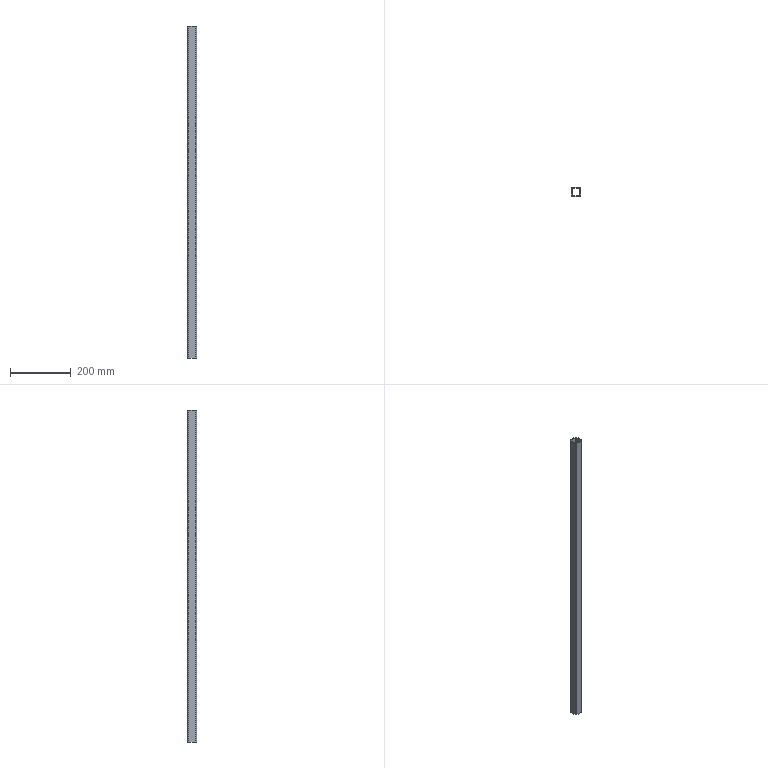Part | SolidWorks | features Attribute 1, ExtruThin 1 | 1 solid | 18 faces | box 30 x 30 x 1098 mm | volume 234556 mm3 | plane 10 | cylinder 8 | commonest cylinder face diameters 4 x4 8 x4
STEP:
#1=CARTESIAN_POINT('',(15.,11.,548.8));
#2=VERTEX_POINT('',#1);
#3=CARTESIAN_POINT('',(11.,15.,548.8));
#4=VERTEX_POINT('',#3);
#5=CARTESIAN_POINT('',(11.,11.,548.8));
#6=DIRECTION('',(0.,0.,1.));
#7=DIRECTION('',(1.,0.,0.));
#8=AXIS2_PLACEMENT_3D('',#5,#6,#7);
#9=CIRCLE('',#8,4.);
#10=EDGE_CURVE('',#2,#4,#9,.T.);
#11=ORIENTED_EDGE('',*,*,#10,.T.);
#12=CARTESIAN_POINT('',(-11.,15.,548.8));
#13=VERTEX_POINT('',#12);
#14=CARTESIAN_POINT('',(11.,15.,548.8));
#15=DIRECTION('',(-1.,0.,0.));
#16=VECTOR('',#15,1000.);
#17=LINE('',#14,#16);
#18=EDGE_CURVE('',#4,#13,#17,.T.);
#19=ORIENTED_EDGE('',*,*,#18,.T.);
#20=CARTESIAN_POINT('',(-15.,11.,548.8));
#21=VERTEX_POINT('',#20);
#22=CARTESIAN_POINT('',(-11.,11.,548.8));
#23=DIRECTION('',(0.,0.,1.));
#24=DIRECTION('',(1.,0.,0.));
#25=AXIS2_PLACEMENT_3D('',#22,#23,#24);
#26=CIRCLE('',#25,4.);
#27=EDGE_CURVE('',#13,#21,#26,.T.);
#28=ORIENTED_EDGE('',*,*,#27,.T.);
#29=CARTESIAN_POINT('',(-15.,-11.,548.8));
#30=VERTEX_POINT('',#29);
#31=CARTESIAN_POINT('',(-15.,-11.,548.8));
#32=DIRECTION('',(0.,1.,0.));
#33=VECTOR('',#32,1000.);
#34=LINE('',#31,#33);
#35=EDGE_CURVE('',#30,#21,#34,.T.);
#36=ORIENTED_EDGE('',*,*,#35,.F.);
#37=CARTESIAN_POINT('',(-11.,-15.,548.8));
#38=VERTEX_POINT('',#37);
#39=CARTESIAN_POINT('',(-11.,-11.,548.8));
#40=DIRECTION('',(0.,0.,1.));
#41=DIRECTION('',(1.,0.,0.));
#42=AXIS2_PLACEMENT_3D('',#39,#40,#41);
#43=CIRCLE('',#42,4.);
#44=EDGE_CURVE('',#30,#38,#43,.T.);
#45=ORIENTED_EDGE('',*,*,#44,.T.);
#46=CARTESIAN_POINT('',(11.,-15.,548.8));
#47=VERTEX_POINT('',#46);
#48=CARTESIAN_POINT('',(-11.,-15.,548.8));
#49=DIRECTION('',(1.,0.,0.));
#50=VECTOR('',#49,1000.);
#51=LINE('',#48,#50);
#52=EDGE_CURVE('',#38,#47,#51,.T.);
#53=ORIENTED_EDGE('',*,*,#52,.T.);
#54=CARTESIAN_POINT('',(15.,-11.,548.8));
#55=VERTEX_POINT('',#54);
#56=CARTESIAN_POINT('',(11.,-11.,548.8));
#57=DIRECTION('',(0.,0.,1.));
#58=DIRECTION('',(1.,0.,0.));
#59=AXIS2_PLACEMENT_3D('',#56,#57,#58);
#60=CIRCLE('',#59,4.);
#61=EDGE_CURVE('',#47,#55,#60,.T.);
#62=ORIENTED_EDGE('',*,*,#61,.T.);
#63=CARTESIAN_POINT('',(15.,11.,548.8));
#64=DIRECTION('',(0.,-1.,0.));
#65=VECTOR('',#64,1000.);
#66=LINE('',#63,#65);
#67=EDGE_CURVE('',#2,#55,#66,.T.);
#68=ORIENTED_EDGE('',*,*,#67,.F.);
#69=EDGE_LOOP('',(#11,#19,#28,#36,#45,#53,#62,#68));
#70=FACE_OUTER_BOUND('',#69,.T.);
#71=CARTESIAN_POINT('',(11.,13.,548.8));
#72=VERTEX_POINT('',#71);
#73=CARTESIAN_POINT('',(-11.,13.,548.8));
#74=VERTEX_POINT('',#73);
#75=CARTESIAN_POINT('',(11.,13.,548.8));
#76=DIRECTION('',(-1.,0.,0.));
#77=VECTOR('',#76,1000.);
#78=LINE('',#75,#77);
#79=EDGE_CURVE('',#72,#74,#78,.T.);
#80=ORIENTED_EDGE('',*,*,#79,.F.);
#81=CARTESIAN_POINT('',(13.,11.,548.8));
#82=VERTEX_POINT('',#81);
#83=CARTESIAN_POINT('',(11.,11.,548.8));
#84=DIRECTION('',(0.,0.,1.));
#85=DIRECTION('',(1.,0.,0.));
#86=AXIS2_PLACEMENT_3D('',#83,#84,#85);
#87=CIRCLE('',#86,2.);
#88=EDGE_CURVE('',#82,#72,#87,.T.);
#89=ORIENTED_EDGE('',*,*,#88,.F.);
#90=CARTESIAN_POINT('',(13.,-11.,548.8));
#91=VERTEX_POINT('',#90);
#92=CARTESIAN_POINT('',(13.,11.,548.8));
#93=DIRECTION('',(0.,-1.,0.));
#94=VECTOR('',#93,1000.);
#95=LINE('',#92,#94);
#96=EDGE_CURVE('',#82,#91,#95,.T.);
#97=ORIENTED_EDGE('',*,*,#96,.T.);
#98=CARTESIAN_POINT('',(11.,-13.,548.8));
#99=VERTEX_POINT('',#98);
#100=CARTESIAN_POINT('',(11.,-11.,548.8));
#101=DIRECTION('',(0.,0.,1.));
#102=DIRECTION('',(1.,0.,0.));
#103=AXIS2_PLACEMENT_3D('',#100,#101,#102);
#104=CIRCLE('',#103,2.);
#105=EDGE_CURVE('',#99,#91,#104,.T.);
#106=ORIENTED_EDGE('',*,*,#105,.F.);
#107=CARTESIAN_POINT('',(-11.,-13.,548.8));
#108=VERTEX_POINT('',#107);
#109=CARTESIAN_POINT('',(-11.,-13.,548.8));
#110=DIRECTION('',(1.,0.,0.));
#111=VECTOR('',#110,1000.);
#112=LINE('',#109,#111);
#113=EDGE_CURVE('',#108,#99,#112,.T.);
#114=ORIENTED_EDGE('',*,*,#113,.F.);
#115=CARTESIAN_POINT('',(-13.,-11.,548.8));
#116=VERTEX_POINT('',#115);
#117=CARTESIAN_POINT('',(-11.,-11.,548.8));
#118=DIRECTION('',(0.,0.,1.));
#119=DIRECTION('',(1.,0.,0.));
#120=AXIS2_PLACEMENT_3D('',#117,#118,#119);
#121=CIRCLE('',#120,2.);
#122=EDGE_CURVE('',#116,#108,#121,.T.);
#123=ORIENTED_EDGE('',*,*,#122,.F.);
#124=CARTESIAN_POINT('',(-13.,11.,548.8));
#125=VERTEX_POINT('',#124);
#126=CARTESIAN_POINT('',(-13.,-11.,548.8));
#127=DIRECTION('',(0.,1.,0.));
#128=VECTOR('',#127,1000.);
#129=LINE('',#126,#128);
#130=EDGE_CURVE('',#116,#125,#129,.T.);
#131=ORIENTED_EDGE('',*,*,#130,.T.);
#132=CARTESIAN_POINT('',(-11.,11.,548.8));
#133=DIRECTION('',(0.,0.,1.));
#134=DIRECTION('',(1.,0.,0.));
#135=AXIS2_PLACEMENT_3D('',#132,#133,#134);
#136=CIRCLE('',#135,2.);
#137=EDGE_CURVE('',#74,#125,#136,.T.);
#138=ORIENTED_EDGE('',*,*,#137,.F.);
#139=EDGE_LOOP('',(#80,#89,#97,#106,#114,#123,#131,#138));
#140=FACE_BOUND('',#139,.T.);
#141=CARTESIAN_POINT('',(11.,11.,548.8));
#142=DIRECTION('',(0.,0.,1.));
#143=DIRECTION('',(1.,0.,0.));
#144=AXIS2_PLACEMENT_3D('',#141,#142,#143);
#145=PLANE('',#144);
#146=ADVANCED_FACE('',(#70,#140),#145,.T.);
#147=CARTESIAN_POINT('',(15.,11.,-548.8));
#148=VERTEX_POINT('',#147);
#149=CARTESIAN_POINT('',(11.,15.,-548.8));
#150=VERTEX_POINT('',#149);
#151=CARTESIAN_POINT('',(11.,11.,-548.8));
#152=DIRECTION('',(0.,0.,1.));
#153=DIRECTION('',(1.,0.,0.));
#154=AXIS2_PLACEMENT_3D('',#151,#152,#153);
#155=CIRCLE('',#154,4.);
#156=EDGE_CURVE('',#148,#150,#155,.T.);
#157=ORIENTED_EDGE('',*,*,#156,.F.);
#158=CARTESIAN_POINT('',(15.,-11.,-548.8));
#159=VERTEX_POINT('',#158);
#160=CARTESIAN_POINT('',(15.,11.,-548.8));
#161=DIRECTION('',(0.,-1.,0.));
#162=VECTOR('',#161,1000.);
#163=LINE('',#160,#162);
#164=EDGE_CURVE('',#148,#159,#163,.T.);
#165=ORIENTED_EDGE('',*,*,#164,.T.);
#166=CARTESIAN_POINT('',(11.,-15.,-548.8));
#167=VERTEX_POINT('',#166);
#168=CARTESIAN_POINT('',(11.,-11.,-548.8));
#169=DIRECTION('',(0.,0.,1.));
#170=DIRECTION('',(1.,0.,0.));
#171=AXIS2_PLACEMENT_3D('',#168,#169,#170);
#172=CIRCLE('',#171,4.);
#173=EDGE_CURVE('',#167,#159,#172,.T.);
#174=ORIENTED_EDGE('',*,*,#173,.F.);
#175=CARTESIAN_POINT('',(-11.,-15.,-548.8));
#176=VERTEX_POINT('',#175);
#177=CARTESIAN_POINT('',(-11.,-15.,-548.8));
#178=DIRECTION('',(1.,0.,0.));
#179=VECTOR('',#178,1000.);
#180=LINE('',#177,#179);
#181=EDGE_CURVE('',#176,#167,#180,.T.);
#182=ORIENTED_EDGE('',*,*,#181,.F.);
#183=CARTESIAN_POINT('',(-15.,-11.,-548.8));
#184=VERTEX_POINT('',#183);
#185=CARTESIAN_POINT('',(-11.,-11.,-548.8));
#186=DIRECTION('',(0.,0.,1.));
#187=DIRECTION('',(1.,0.,0.));
#188=AXIS2_PLACEMENT_3D('',#185,#186,#187);
#189=CIRCLE('',#188,4.);
#190=EDGE_CURVE('',#184,#176,#189,.T.);
#191=ORIENTED_EDGE('',*,*,#190,.F.);
#192=CARTESIAN_POINT('',(-15.,11.,-548.8));
#193=VERTEX_POINT('',#192);
#194=CARTESIAN_POINT('',(-15.,-11.,-548.8));
#195=DIRECTION('',(0.,1.,0.));
#196=VECTOR('',#195,1000.);
#197=LINE('',#194,#196);
#198=EDGE_CURVE('',#184,#193,#197,.T.);
#199=ORIENTED_EDGE('',*,*,#198,.T.);
#200=CARTESIAN_POINT('',(-11.,15.,-548.8));
#201=VERTEX_POINT('',#200);
#202=CARTESIAN_POINT('',(-11.,11.,-548.8));
#203=DIRECTION('',(0.,0.,1.));
#204=DIRECTION('',(1.,0.,0.));
#205=AXIS2_PLACEMENT_3D('',#202,#203,#204);
#206=CIRCLE('',#205,4.);
#207=EDGE_CURVE('',#201,#193,#206,.T.);
#208=ORIENTED_EDGE('',*,*,#207,.F.);
#209=CARTESIAN_POINT('',(11.,15.,-548.8));
#210=DIRECTION('',(-1.,0.,0.));
#211=VECTOR('',#210,1000.);
#212=LINE('',#209,#211);
#213=EDGE_CURVE('',#150,#201,#212,.T.);
#214=ORIENTED_EDGE('',*,*,#213,.F.);
#215=EDGE_LOOP('',(#157,#165,#174,#182,#191,#199,#208,#214));
#216=FACE_OUTER_BOUND('',#215,.T.);
#217=CARTESIAN_POINT('',(13.,11.,-548.8));
#218=VERTEX_POINT('',#217);
#219=CARTESIAN_POINT('',(11.,13.,-548.8));
#220=VERTEX_POINT('',#219);
#221=CARTESIAN_POINT('',(11.,11.,-548.8));
#222=DIRECTION('',(0.,0.,1.));
#223=DIRECTION('',(1.,0.,0.));
#224=AXIS2_PLACEMENT_3D('',#221,#222,#223);
#225=CIRCLE('',#224,2.);
#226=EDGE_CURVE('',#218,#220,#225,.T.);
#227=ORIENTED_EDGE('',*,*,#226,.T.);
#228=CARTESIAN_POINT('',(-11.,13.,-548.8));
#229=VERTEX_POINT('',#228);
#230=CARTESIAN_POINT('',(11.,13.,-548.8));
#231=DIRECTION('',(-1.,0.,0.));
#232=VECTOR('',#231,1000.);
#233=LINE('',#230,#232);
#234=EDGE_CURVE('',#220,#229,#233,.T.);
#235=ORIENTED_EDGE('',*,*,#234,.T.);
#236=CARTESIAN_POINT('',(-13.,11.,-548.8));
#237=VERTEX_POINT('',#236);
#238=CARTESIAN_POINT('',(-11.,11.,-548.8));
#239=DIRECTION('',(0.,0.,1.));
#240=DIRECTION('',(1.,0.,0.));
#241=AXIS2_PLACEMENT_3D('',#238,#239,#240);
#242=CIRCLE('',#241,2.);
#243=EDGE_CURVE('',#229,#237,#242,.T.);
#244=ORIENTED_EDGE('',*,*,#243,.T.);
#245=CARTESIAN_POINT('',(-13.,-11.,-548.8));
#246=VERTEX_POINT('',#245);
#247=CARTESIAN_POINT('',(-13.,-11.,-548.8));
#248=DIRECTION('',(0.,1.,0.));
#249=VECTOR('',#248,1000.);
#250=LINE('',#247,#249);
#251=EDGE_CURVE('',#246,#237,#250,.T.);
#252=ORIENTED_EDGE('',*,*,#251,.F.);
#253=CARTESIAN_POINT('',(-11.,-13.,-548.8));
#254=VERTEX_POINT('',#253);
#255=CARTESIAN_POINT('',(-11.,-11.,-548.8));
#256=DIRECTION('',(0.,0.,1.));
#257=DIRECTION('',(1.,0.,0.));
#258=AXIS2_PLACEMENT_3D('',#255,#256,#257);
#259=CIRCLE('',#258,2.);
#260=EDGE_CURVE('',#246,#254,#259,.T.);
#261=ORIENTED_EDGE('',*,*,#260,.T.);
#262=CARTESIAN_POINT('',(11.,-13.,-548.8));
#263=VERTEX_POINT('',#262);
#264=CARTESIAN_POINT('',(-11.,-13.,-548.8));
#265=DIRECTION('',(1.,0.,0.));
#266=VECTOR('',#265,1000.);
#267=LINE('',#264,#266);
#268=EDGE_CURVE('',#254,#263,#267,.T.);
#269=ORIENTED_EDGE('',*,*,#268,.T.);
#270=CARTESIAN_POINT('',(13.,-11.,-548.8));
#271=VERTEX_POINT('',#270);
#272=CARTESIAN_POINT('',(11.,-11.,-548.8));
#273=DIRECTION('',(0.,0.,1.));
#274=DIRECTION('',(1.,0.,0.));
#275=AXIS2_PLACEMENT_3D('',#272,#273,#274);
#276=CIRCLE('',#275,2.);
#277=EDGE_CURVE('',#263,#271,#276,.T.);
#278=ORIENTED_EDGE('',*,*,#277,.T.);
#279=CARTESIAN_POINT('',(13.,11.,-548.8));
#280=DIRECTION('',(0.,-1.,0.));
#281=VECTOR('',#280,1000.);
#282=LINE('',#279,#281);
#283=EDGE_CURVE('',#218,#271,#282,.T.);
#284=ORIENTED_EDGE('',*,*,#283,.F.);
#285=EDGE_LOOP('',(#227,#235,#244,#252,#261,#269,#278,#284));
#286=FACE_BOUND('',#285,.T.);
#287=CARTESIAN_POINT('',(11.,11.,-548.8));
#288=DIRECTION('',(0.,0.,1.));
#289=DIRECTION('',(1.,0.,0.));
#290=AXIS2_PLACEMENT_3D('',#287,#288,#289);
#291=PLANE('',#290);
#292=ADVANCED_FACE('',(#216,#286),#291,.F.);
#293=ORIENTED_EDGE('',*,*,#156,.T.);
#294=CARTESIAN_POINT('',(11.,15.,548.8));
#295=DIRECTION('',(0.,0.,-1.));
#296=VECTOR('',#295,1000.);
#297=LINE('',#294,#296);
#298=EDGE_CURVE('',#4,#150,#297,.T.);
#299=ORIENTED_EDGE('',*,*,#298,.F.);
#300=ORIENTED_EDGE('',*,*,#10,.F.);
#301=CARTESIAN_POINT('',(15.,11.,548.8));
#302=DIRECTION('',(0.,0.,-1.));
#303=VECTOR('',#302,1000.);
#304=LINE('',#301,#303);
#305=EDGE_CURVE('',#2,#148,#304,.T.);
#306=ORIENTED_EDGE('',*,*,#305,.T.);
#307=EDGE_LOOP('',(#293,#299,#300,#306));
#308=FACE_OUTER_BOUND('',#307,.T.);
#309=CARTESIAN_POINT('',(11.,11.,548.8));
#310=DIRECTION('',(0.,0.,-1.));
#311=DIRECTION('',(-1.,0.,0.));
#312=AXIS2_PLACEMENT_3D('',#309,#310,#311);
#313=CYLINDRICAL_SURFACE('',#312,4.);
#314=ADVANCED_FACE('',(#308),#313,.T.);
#315=ORIENTED_EDGE('',*,*,#213,.T.);
#316=CARTESIAN_POINT('',(-11.,15.,548.8));
#317=DIRECTION('',(0.,0.,-1.));
#318=VECTOR('',#317,1000.);
#319=LINE('',#316,#318);
#320=EDGE_CURVE('',#13,#201,#319,.T.);
#321=ORIENTED_EDGE('',*,*,#320,.F.);
#322=ORIENTED_EDGE('',*,*,#18,.F.);
#323=ORIENTED_EDGE('',*,*,#298,.T.);
#324=EDGE_LOOP('',(#315,#321,#322,#323));
#325=FACE_OUTER_BOUND('',#324,.T.);
#326=CARTESIAN_POINT('',(11.,15.,548.8));
#327=DIRECTION('',(0.,-1.,0.));
#328=DIRECTION('',(0.,0.,-1.));
#329=AXIS2_PLACEMENT_3D('',#326,#327,#328);
#330=PLANE('',#329);
#331=ADVANCED_FACE('',(#325),#330,.F.);
#332=ORIENTED_EDGE('',*,*,#207,.T.);
#333=CARTESIAN_POINT('',(-15.,11.,548.8));
#334=DIRECTION('',(0.,0.,-1.));
#335=VECTOR('',#334,1000.);
#336=LINE('',#333,#335);
#337=EDGE_CURVE('',#21,#193,#336,.T.);
#338=ORIENTED_EDGE('',*,*,#337,.F.);
#339=ORIENTED_EDGE('',*,*,#27,.F.);
#340=ORIENTED_EDGE('',*,*,#320,.T.);
#341=EDGE_LOOP('',(#332,#338,#339,#340));
#342=FACE_OUTER_BOUND('',#341,.T.);
#343=CARTESIAN_POINT('',(-11.,11.,548.8));
#344=DIRECTION('',(0.,0.,-1.));
#345=DIRECTION('',(-1.,0.,0.));
#346=AXIS2_PLACEMENT_3D('',#343,#344,#345);
#347=CYLINDRICAL_SURFACE('',#346,4.);
#348=ADVANCED_FACE('',(#342),#347,.T.);
#349=ORIENTED_EDGE('',*,*,#198,.F.);
#350=CARTESIAN_POINT('',(-15.,-11.,548.8));
#351=DIRECTION('',(0.,0.,-1.));
#352=VECTOR('',#351,1000.);
#353=LINE('',#350,#352);
#354=EDGE_CURVE('',#30,#184,#353,.T.);
#355=ORIENTED_EDGE('',*,*,#354,.F.);
#356=ORIENTED_EDGE('',*,*,#35,.T.);
#357=ORIENTED_EDGE('',*,*,#337,.T.);
#358=EDGE_LOOP('',(#349,#355,#356,#357));
#359=FACE_OUTER_BOUND('',#358,.T.);
#360=CARTESIAN_POINT('',(-15.,-11.,548.8));
#361=DIRECTION('',(-1.,0.,0.));
#362=DIRECTION('',(0.,0.,1.));
#363=AXIS2_PLACEMENT_3D('',#360,#361,#362);
#364=PLANE('',#363);
#365=ADVANCED_FACE('',(#359),#364,.T.);
#366=ORIENTED_EDGE('',*,*,#190,.T.);
#367=CARTESIAN_POINT('',(-11.,-15.,548.8));
#368=DIRECTION('',(0.,0.,-1.));
#369=VECTOR('',#368,1000.);
#370=LINE('',#367,#369);
#371=EDGE_CURVE('',#38,#176,#370,.T.);
#372=ORIENTED_EDGE('',*,*,#371,.F.);
#373=ORIENTED_EDGE('',*,*,#44,.F.);
#374=ORIENTED_EDGE('',*,*,#354,.T.);
#375=EDGE_LOOP('',(#366,#372,#373,#374));
#376=FACE_OUTER_BOUND('',#375,.T.);
#377=CARTESIAN_POINT('',(-11.,-11.,548.8));
#378=DIRECTION('',(0.,0.,-1.));
#379=DIRECTION('',(-1.,0.,0.));
#380=AXIS2_PLACEMENT_3D('',#377,#378,#379);
#381=CYLINDRICAL_SURFACE('',#380,4.);
#382=ADVANCED_FACE('',(#376),#381,.T.);
#383=ORIENTED_EDGE('',*,*,#181,.T.);
#384=CARTESIAN_POINT('',(11.,-15.,548.8));
#385=DIRECTION('',(0.,0.,-1.));
#386=VECTOR('',#385,1000.);
#387=LINE('',#384,#386);
#388=EDGE_CURVE('',#47,#167,#387,.T.);
#389=ORIENTED_EDGE('',*,*,#388,.F.);
#390=ORIENTED_EDGE('',*,*,#52,.F.);
#391=ORIENTED_EDGE('',*,*,#371,.T.);
#392=EDGE_LOOP('',(#383,#389,#390,#391));
#393=FACE_OUTER_BOUND('',#392,.T.);
#394=CARTESIAN_POINT('',(-11.,-15.,548.8));
#395=DIRECTION('',(0.,1.,0.));
#396=DIRECTION('',(0.,0.,1.));
#397=AXIS2_PLACEMENT_3D('',#394,#395,#396);
#398=PLANE('',#397);
#399=ADVANCED_FACE('',(#393),#398,.F.);
#400=ORIENTED_EDGE('',*,*,#173,.T.);
#401=CARTESIAN_POINT('',(15.,-11.,548.8));
#402=DIRECTION('',(0.,0.,-1.));
#403=VECTOR('',#402,1000.);
#404=LINE('',#401,#403);
#405=EDGE_CURVE('',#55,#159,#404,.T.);
#406=ORIENTED_EDGE('',*,*,#405,.F.);
#407=ORIENTED_EDGE('',*,*,#61,.F.);
#408=ORIENTED_EDGE('',*,*,#388,.T.);
#409=EDGE_LOOP('',(#400,#406,#407,#408));
#410=FACE_OUTER_BOUND('',#409,.T.);
#411=CARTESIAN_POINT('',(11.,-11.,548.8));
#412=DIRECTION('',(0.,0.,-1.));
#413=DIRECTION('',(-1.,0.,0.));
#414=AXIS2_PLACEMENT_3D('',#411,#412,#413);
#415=CYLINDRICAL_SURFACE('',#414,4.);
#416=ADVANCED_FACE('',(#410),#415,.T.);
#417=ORIENTED_EDGE('',*,*,#164,.F.);
#418=ORIENTED_EDGE('',*,*,#305,.F.);
#419=ORIENTED_EDGE('',*,*,#67,.T.);
#420=ORIENTED_EDGE('',*,*,#405,.T.);
#421=EDGE_LOOP('',(#417,#418,#419,#420));
#422=FACE_OUTER_BOUND('',#421,.T.);
#423=CARTESIAN_POINT('',(15.,11.,548.8));
#424=DIRECTION('',(1.,0.,0.));
#425=DIRECTION('',(0.,0.,-1.));
#426=AXIS2_PLACEMENT_3D('',#423,#424,#425);
#427=PLANE('',#426);
#428=ADVANCED_FACE('',(#422),#427,.T.);
#429=ORIENTED_EDGE('',*,*,#226,.F.);
#430=CARTESIAN_POINT('',(13.,11.,548.8));
#431=DIRECTION('',(0.,0.,-1.));
#432=VECTOR('',#431,1000.);
#433=LINE('',#430,#432);
#434=EDGE_CURVE('',#82,#218,#433,.T.);
#435=ORIENTED_EDGE('',*,*,#434,.F.);
#436=ORIENTED_EDGE('',*,*,#88,.T.);
#437=CARTESIAN_POINT('',(11.,13.,548.8));
#438=DIRECTION('',(0.,0.,-1.));
#439=VECTOR('',#438,1000.);
#440=LINE('',#437,#439);
#441=EDGE_CURVE('',#72,#220,#440,.T.);
#442=ORIENTED_EDGE('',*,*,#441,.T.);
#443=EDGE_LOOP('',(#429,#435,#436,#442));
#444=FACE_OUTER_BOUND('',#443,.T.);
#445=CARTESIAN_POINT('',(11.,11.,548.8));
#446=DIRECTION('',(0.,0.,-1.));
#447=DIRECTION('',(-1.,0.,0.));
#448=AXIS2_PLACEMENT_3D('',#445,#446,#447);
#449=CYLINDRICAL_SURFACE('',#448,2.);
#450=ADVANCED_FACE('',(#444),#449,.F.);
#451=ORIENTED_EDGE('',*,*,#234,.F.);
#452=ORIENTED_EDGE('',*,*,#441,.F.);
#453=ORIENTED_EDGE('',*,*,#79,.T.);
#454=CARTESIAN_POINT('',(-11.,13.,548.8));
#455=DIRECTION('',(0.,0.,-1.));
#456=VECTOR('',#455,1000.);
#457=LINE('',#454,#456);
#458=EDGE_CURVE('',#74,#229,#457,.T.);
#459=ORIENTED_EDGE('',*,*,#458,.T.);
#460=EDGE_LOOP('',(#451,#452,#453,#459));
#461=FACE_OUTER_BOUND('',#460,.T.);
#462=CARTESIAN_POINT('',(11.,13.,548.8));
#463=DIRECTION('',(0.,-1.,0.));
#464=DIRECTION('',(0.,0.,-1.));
#465=AXIS2_PLACEMENT_3D('',#462,#463,#464);
#466=PLANE('',#465);
#467=ADVANCED_FACE('',(#461),#466,.T.);
#468=ORIENTED_EDGE('',*,*,#243,.F.);
#469=ORIENTED_EDGE('',*,*,#458,.F.);
#470=ORIENTED_EDGE('',*,*,#137,.T.);
#471=CARTESIAN_POINT('',(-13.,11.,548.8));
#472=DIRECTION('',(0.,0.,-1.));
#473=VECTOR('',#472,1000.);
#474=LINE('',#471,#473);
#475=EDGE_CURVE('',#125,#237,#474,.T.);
#476=ORIENTED_EDGE('',*,*,#475,.T.);
#477=EDGE_LOOP('',(#468,#469,#470,#476));
#478=FACE_OUTER_BOUND('',#477,.T.);
#479=CARTESIAN_POINT('',(-11.,11.,548.8));
#480=DIRECTION('',(0.,0.,-1.));
#481=DIRECTION('',(-1.,0.,0.));
#482=AXIS2_PLACEMENT_3D('',#479,#480,#481);
#483=CYLINDRICAL_SURFACE('',#482,2.);
#484=ADVANCED_FACE('',(#478),#483,.F.);
#485=ORIENTED_EDGE('',*,*,#251,.T.);
#486=ORIENTED_EDGE('',*,*,#475,.F.);
#487=ORIENTED_EDGE('',*,*,#130,.F.);
#488=CARTESIAN_POINT('',(-13.,-11.,548.8));
#489=DIRECTION('',(0.,0.,-1.));
#490=VECTOR('',#489,1000.);
#491=LINE('',#488,#490);
#492=EDGE_CURVE('',#116,#246,#491,.T.);
#493=ORIENTED_EDGE('',*,*,#492,.T.);
#494=EDGE_LOOP('',(#485,#486,#487,#493));
#495=FACE_OUTER_BOUND('',#494,.T.);
#496=CARTESIAN_POINT('',(-13.,-11.,548.8));
#497=DIRECTION('',(-1.,0.,0.));
#498=DIRECTION('',(0.,0.,1.));
#499=AXIS2_PLACEMENT_3D('',#496,#497,#498);
#500=PLANE('',#499);
#501=ADVANCED_FACE('',(#495),#500,.F.);
#502=ORIENTED_EDGE('',*,*,#260,.F.);
#503=ORIENTED_EDGE('',*,*,#492,.F.);
#504=ORIENTED_EDGE('',*,*,#122,.T.);
#505=CARTESIAN_POINT('',(-11.,-13.,548.8));
#506=DIRECTION('',(0.,0.,-1.));
#507=VECTOR('',#506,1000.);
#508=LINE('',#505,#507);
#509=EDGE_CURVE('',#108,#254,#508,.T.);
#510=ORIENTED_EDGE('',*,*,#509,.T.);
#511=EDGE_LOOP('',(#502,#503,#504,#510));
#512=FACE_OUTER_BOUND('',#511,.T.);
#513=CARTESIAN_POINT('',(-11.,-11.,548.8));
#514=DIRECTION('',(0.,0.,-1.));
#515=DIRECTION('',(-1.,0.,0.));
#516=AXIS2_PLACEMENT_3D('',#513,#514,#515);
#517=CYLINDRICAL_SURFACE('',#516,2.);
#518=ADVANCED_FACE('',(#512),#517,.F.);
#519=ORIENTED_EDGE('',*,*,#268,.F.);
#520=ORIENTED_EDGE('',*,*,#509,.F.);
#521=ORIENTED_EDGE('',*,*,#113,.T.);
#522=CARTESIAN_POINT('',(11.,-13.,548.8));
#523=DIRECTION('',(0.,0.,-1.));
#524=VECTOR('',#523,1000.);
#525=LINE('',#522,#524);
#526=EDGE_CURVE('',#99,#263,#525,.T.);
#527=ORIENTED_EDGE('',*,*,#526,.T.);
#528=EDGE_LOOP('',(#519,#520,#521,#527));
#529=FACE_OUTER_BOUND('',#528,.T.);
#530=CARTESIAN_POINT('',(-11.,-13.,548.8));
#531=DIRECTION('',(0.,1.,0.));
#532=DIRECTION('',(0.,0.,1.));
#533=AXIS2_PLACEMENT_3D('',#530,#531,#532);
#534=PLANE('',#533);
#535=ADVANCED_FACE('',(#529),#534,.T.);
#536=ORIENTED_EDGE('',*,*,#277,.F.);
#537=ORIENTED_EDGE('',*,*,#526,.F.);
#538=ORIENTED_EDGE('',*,*,#105,.T.);
#539=CARTESIAN_POINT('',(13.,-11.,548.8));
#540=DIRECTION('',(0.,0.,-1.));
#541=VECTOR('',#540,1000.);
#542=LINE('',#539,#541);
#543=EDGE_CURVE('',#91,#271,#542,.T.);
#544=ORIENTED_EDGE('',*,*,#543,.T.);
#545=EDGE_LOOP('',(#536,#537,#538,#544));
#546=FACE_OUTER_BOUND('',#545,.T.);
#547=CARTESIAN_POINT('',(11.,-11.,548.8));
#548=DIRECTION('',(0.,0.,-1.));
#549=DIRECTION('',(-1.,0.,0.));
#550=AXIS2_PLACEMENT_3D('',#547,#548,#549);
#551=CYLINDRICAL_SURFACE('',#550,2.);
#552=ADVANCED_FACE('',(#546),#551,.F.);
#553=ORIENTED_EDGE('',*,*,#283,.T.);
#554=ORIENTED_EDGE('',*,*,#543,.F.);
#555=ORIENTED_EDGE('',*,*,#96,.F.);
#556=ORIENTED_EDGE('',*,*,#434,.T.);
#557=EDGE_LOOP('',(#553,#554,#555,#556));
#558=FACE_OUTER_BOUND('',#557,.T.);
#559=CARTESIAN_POINT('',(13.,11.,548.8));
#560=DIRECTION('',(1.,0.,0.));
#561=DIRECTION('',(0.,0.,-1.));
#562=AXIS2_PLACEMENT_3D('',#559,#560,#561);
#563=PLANE('',#562);
#564=ADVANCED_FACE('',(#558),#563,.F.);
#565=CLOSED_SHELL('',(#146,#292,#314,#331,#348,#365,#382,#399,#416,#428,#450,#467,#484,#501,#518,#535,#552,#564));
#566=MANIFOLD_SOLID_BREP('',#565);
#567=CARTESIAN_POINT('',(0.,0.,0.));
#568=DIRECTION('',(0.,0.,1.));
#569=DIRECTION('',(1.,0.,0.));
#570=AXIS2_PLACEMENT_3D('',#567,#568,#569);
#571=(LENGTH_UNIT()NAMED_UNIT(*)SI_UNIT(.MILLI.,.METRE.));
#572=UNCERTAINTY_MEASURE_WITH_UNIT(LENGTH_MEASURE(0.00001),#571,'','');
#573=(NAMED_UNIT(*)PLANE_ANGLE_UNIT()SI_UNIT($,.RADIAN.));
#574=(NAMED_UNIT(*)SI_UNIT($,.STERADIAN.)SOLID_ANGLE_UNIT());
#575=(GEOMETRIC_REPRESENTATION_CONTEXT(3)GLOBAL_UNCERTAINTY_ASSIGNED_CONTEXT((#572))GLOBAL_UNIT_ASSIGNED_CONTEXT((#571,#573,#574))REPRESENTATION_CONTEXT('',''));
#576=ADVANCED_BREP_SHAPE_REPRESENTATION('',(#566,#570),#575);